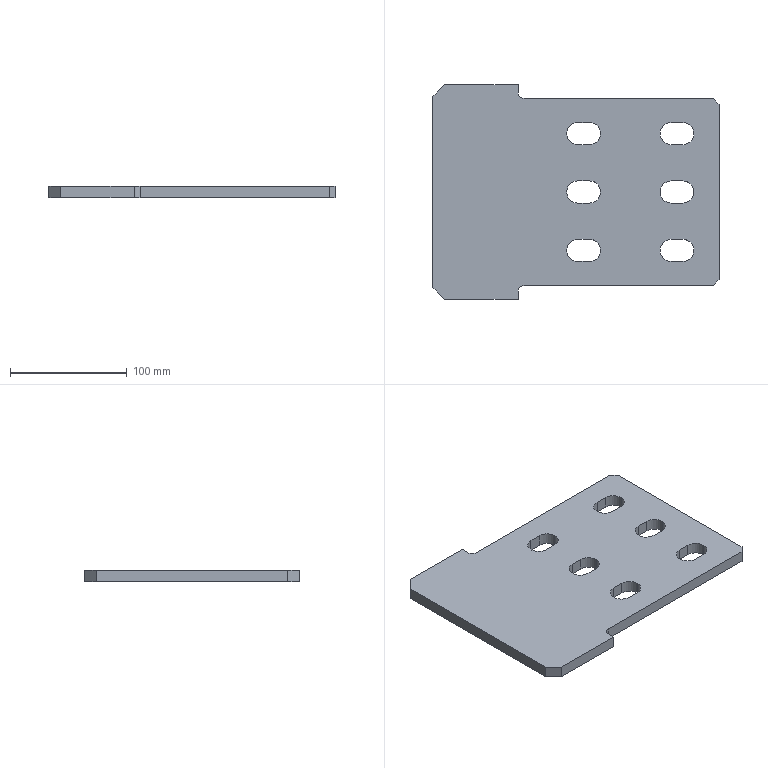Part | STEP file | 筋Plate-200×100-200-30度 | 1 solid | 46 faces | box 245 x 184 x 10 mm | volume 379966 mm3 | plane 26 | cylinder 20 | commonest cylinder face diameters 19 x18 10 x2